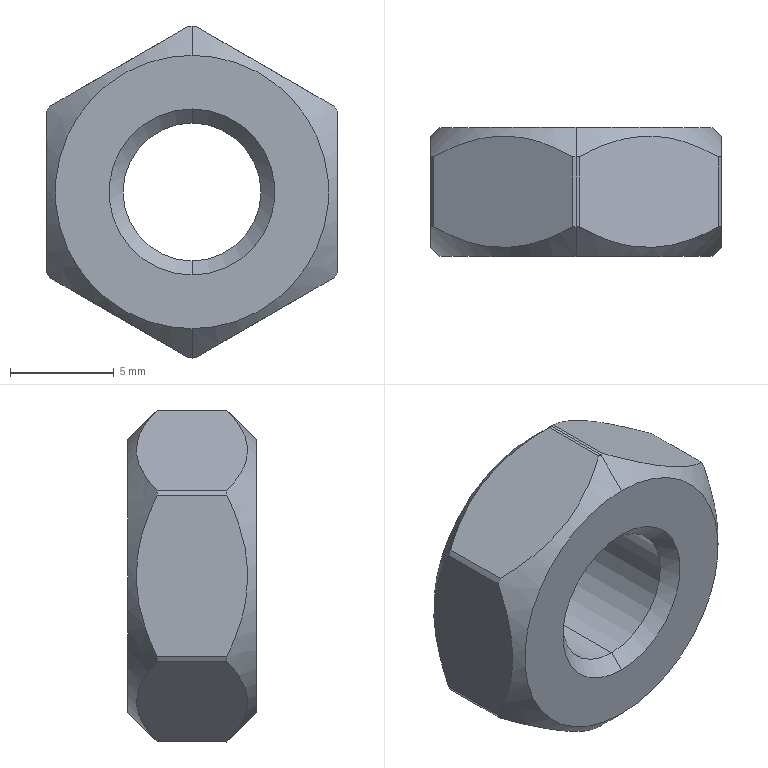Part | SolidWorks | features BaseBody 1 | 1 solid | 23 faces | box 14 x 6.2 x 16 mm | volume 801.096 mm3 | cylinder 9 | plane 8 | cone 6 | commonest cylinder face diameters 16 x7 6.647 x2
STEP:
#1=CARTESIAN_POINT('',(0.,28.776,-3.324));
#2=VERTEX_POINT('',#1);
#3=CARTESIAN_POINT('',(0.,28.776,3.324));
#4=VERTEX_POINT('',#3);
#5=CARTESIAN_POINT('',(0.,28.776,0.));
#6=DIRECTION('',(0.,1.,0.));
#7=DIRECTION('',(0.,0.,1.));
#8=AXIS2_PLACEMENT_3D('',#5,#6,#7);
#9=CIRCLE('',#8,3.324);
#10=EDGE_CURVE('',#2,#4,#9,.T.);
#11=ORIENTED_EDGE('',*,*,#10,.F.);
#12=CARTESIAN_POINT('',(0.,34.3,-3.324));
#13=VERTEX_POINT('',#12);
#14=CARTESIAN_POINT('',(0.,34.3,-3.324));
#15=DIRECTION('',(0.,1.,0.));
#16=VECTOR('',#15,1000.);
#17=LINE('',#14,#16);
#18=EDGE_CURVE('',#2,#13,#17,.T.);
#19=ORIENTED_EDGE('',*,*,#18,.T.);
#20=CARTESIAN_POINT('',(0.,34.3,3.324));
#21=VERTEX_POINT('',#20);
#22=CARTESIAN_POINT('',(0.,34.3,0.));
#23=DIRECTION('',(0.,-1.,0.));
#24=DIRECTION('',(0.,0.,1.));
#25=AXIS2_PLACEMENT_3D('',#22,#23,#24);
#26=CIRCLE('',#25,3.324);
#27=EDGE_CURVE('',#21,#13,#26,.T.);
#28=ORIENTED_EDGE('',*,*,#27,.F.);
#29=CARTESIAN_POINT('',(0.,34.3,3.324));
#30=DIRECTION('',(0.,1.,0.));
#31=VECTOR('',#30,1000.);
#32=LINE('',#29,#31);
#33=EDGE_CURVE('',#4,#21,#32,.T.);
#34=ORIENTED_EDGE('',*,*,#33,.F.);
#35=EDGE_LOOP('',(#11,#19,#28,#34));
#36=FACE_OUTER_BOUND('',#35,.T.);
#37=CARTESIAN_POINT('',(0.,34.3,0.));
#38=DIRECTION('',(0.,1.,0.));
#39=DIRECTION('',(0.,0.,1.));
#40=AXIS2_PLACEMENT_3D('',#37,#38,#39);
#41=CYLINDRICAL_SURFACE('',#40,3.324);
#42=ADVANCED_FACE('',(#36),#41,.F.);
#43=ORIENTED_EDGE('',*,*,#10,.T.);
#44=CARTESIAN_POINT('',(0.,28.1,4.));
#45=VERTEX_POINT('',#44);
#46=CARTESIAN_POINT('',(0.,28.1,4.));
#47=DIRECTION('',(0.,-0.7071,0.7071));
#48=VECTOR('',#47,1000.);
#49=LINE('',#46,#48);
#50=EDGE_CURVE('',#4,#45,#49,.T.);
#51=ORIENTED_EDGE('',*,*,#50,.T.);
#52=CARTESIAN_POINT('',(0.,28.1,-4.));
#53=VERTEX_POINT('',#52);
#54=CARTESIAN_POINT('',(0.,28.1,0.));
#55=DIRECTION('',(0.,1.,0.));
#56=DIRECTION('',(0.,0.,-1.));
#57=AXIS2_PLACEMENT_3D('',#54,#55,#56);
#58=CIRCLE('',#57,4.);
#59=EDGE_CURVE('',#53,#45,#58,.T.);
#60=ORIENTED_EDGE('',*,*,#59,.F.);
#61=CARTESIAN_POINT('',(0.,28.1,-4.));
#62=DIRECTION('',(0.,-0.7071,-0.7071));
#63=VECTOR('',#62,1000.);
#64=LINE('',#61,#63);
#65=EDGE_CURVE('',#2,#53,#64,.T.);
#66=ORIENTED_EDGE('',*,*,#65,.F.);
#67=EDGE_LOOP('',(#43,#51,#60,#66));
#68=FACE_OUTER_BOUND('',#67,.T.);
#69=CARTESIAN_POINT('',(0.,28.1,0.));
#70=DIRECTION('',(0.,-1.,0.));
#71=DIRECTION('',(0.,0.,-1.));
#72=AXIS2_PLACEMENT_3D('',#69,#70,#71);
#73=CONICAL_SURFACE('',#72,4.,0.7854);
#74=ADVANCED_FACE('',(#68),#73,.F.);
#75=CARTESIAN_POINT('',(0.,34.3,-6.586));
#76=VERTEX_POINT('',#75);
#77=CARTESIAN_POINT('',(0.,34.3,6.586));
#78=VERTEX_POINT('',#77);
#79=CARTESIAN_POINT('',(0.,34.3,0.));
#80=DIRECTION('',(0.,-1.,0.));
#81=DIRECTION('',(0.,0.,-1.));
#82=AXIS2_PLACEMENT_3D('',#79,#80,#81);
#83=CIRCLE('',#82,6.586);
#84=EDGE_CURVE('',#76,#78,#83,.T.);
#85=ORIENTED_EDGE('',*,*,#84,.T.);
#86=CARTESIAN_POINT('',(0.,32.886,8.));
#87=VERTEX_POINT('',#86);
#88=CARTESIAN_POINT('',(0.,32.886,8.));
#89=DIRECTION('',(0.,-0.7071,0.7071));
#90=VECTOR('',#89,1000.);
#91=LINE('',#88,#90);
#92=EDGE_CURVE('',#78,#87,#91,.T.);
#93=ORIENTED_EDGE('',*,*,#92,.T.);
#94=CARTESIAN_POINT('',(0.1459,32.886,7.999));
#95=VERTEX_POINT('',#94);
#96=CARTESIAN_POINT('',(0.,32.886,0.));
#97=DIRECTION('',(0.,-1.,0.));
#98=DIRECTION('',(0.,0.,1.));
#99=AXIS2_PLACEMENT_3D('',#96,#97,#98);
#100=CIRCLE('',#99,8.);
#101=EDGE_CURVE('',#95,#87,#100,.T.);
#102=ORIENTED_EDGE('',*,*,#101,.F.);
#103=CARTESIAN_POINT('',(6.854,32.886,4.126));
#104=VERTEX_POINT('',#103);
#105=CARTESIAN_POINT('',(0.1459,32.886,7.999));
#106=CARTESIAN_POINT('',(0.672,33.18,7.695));
#107=CARTESIAN_POINT('',(1.21,33.428,7.385));
#108=CARTESIAN_POINT('',(2.043,33.693,6.903));
#109=CARTESIAN_POINT('',(2.325,33.763,6.74));
#110=CARTESIAN_POINT('',(2.901,33.859,6.408));
#111=CARTESIAN_POINT('',(3.197,33.885,6.237));
#112=CARTESIAN_POINT('',(4.073,33.887,5.731));
#113=CARTESIAN_POINT('',(4.647,33.789,5.4));
#114=CARTESIAN_POINT('',(5.496,33.523,4.91));
#115=CARTESIAN_POINT('',(5.775,33.415,4.749));
#116=CARTESIAN_POINT('',(6.321,33.17,4.433));
#117=CARTESIAN_POINT('',(6.59,33.034,4.278));
#118=CARTESIAN_POINT('',(6.854,32.886,4.126));
#119=B_SPLINE_CURVE_WITH_KNOTS('',3,(#105,#106,#107,#108,#109,#110,#111,#112,#113,#114,#115,#116,#117,#118),.UNSPECIFIED.,.F.,.F.,(4,2,2,2,2,2,4),(0.,0.001996,0.002994,0.003992,0.005988,0.006986,0.007984),.UNSPECIFIED.);
#120=EDGE_CURVE('',#95,#104,#119,.T.);
#121=ORIENTED_EDGE('',*,*,#120,.T.);
#122=CARTESIAN_POINT('',(7.,32.886,3.873));
#123=VERTEX_POINT('',#122);
#124=CARTESIAN_POINT('',(0.,32.886,0.));
#125=DIRECTION('',(0.,-1.,0.));
#126=DIRECTION('',(0.,0.,1.));
#127=AXIS2_PLACEMENT_3D('',#124,#125,#126);
#128=CIRCLE('',#127,8.);
#129=EDGE_CURVE('',#123,#104,#128,.T.);
#130=ORIENTED_EDGE('',*,*,#129,.F.);
#131=CARTESIAN_POINT('',(7.,32.886,-3.873));
#132=VERTEX_POINT('',#131);
#133=CARTESIAN_POINT('',(7.,32.886,3.873));
#134=CARTESIAN_POINT('',(7.,33.18,3.265));
#135=CARTESIAN_POINT('',(7.,33.428,2.645));
#136=CARTESIAN_POINT('',(7.,33.693,1.682));
#137=CARTESIAN_POINT('',(7.,33.763,1.356));
#138=CARTESIAN_POINT('',(7.,33.859,0.6915));
#139=CARTESIAN_POINT('',(7.,33.885,0.3497));
#140=CARTESIAN_POINT('',(7.,33.887,-0.6617));
#141=CARTESIAN_POINT('',(7.,33.789,-1.325));
#142=CARTESIAN_POINT('',(7.,33.523,-2.305));
#143=CARTESIAN_POINT('',(7.,33.415,-2.627));
#144=CARTESIAN_POINT('',(7.,33.17,-3.258));
#145=CARTESIAN_POINT('',(7.,33.034,-3.568));
#146=CARTESIAN_POINT('',(7.,32.886,-3.873));
#147=B_SPLINE_CURVE_WITH_KNOTS('',3,(#133,#134,#135,#136,#137,#138,#139,#140,#141,#142,#143,#144,#145,#146),.UNSPECIFIED.,.F.,.F.,(4,2,2,2,2,2,4),(0.,0.001996,0.002994,0.003992,0.005988,0.006986,0.007984),.UNSPECIFIED.);
#148=EDGE_CURVE('',#123,#132,#147,.T.);
#149=ORIENTED_EDGE('',*,*,#148,.T.);
#150=CARTESIAN_POINT('',(6.854,32.886,-4.126));
#151=VERTEX_POINT('',#150);
#152=CARTESIAN_POINT('',(0.,32.886,0.));
#153=DIRECTION('',(0.,-1.,0.));
#154=DIRECTION('',(0.,0.,1.));
#155=AXIS2_PLACEMENT_3D('',#152,#153,#154);
#156=CIRCLE('',#155,8.);
#157=EDGE_CURVE('',#151,#132,#156,.T.);
#158=ORIENTED_EDGE('',*,*,#157,.F.);
#159=CARTESIAN_POINT('',(0.1459,32.886,-7.999));
#160=VERTEX_POINT('',#159);
#161=CARTESIAN_POINT('',(6.854,32.886,-4.126));
#162=CARTESIAN_POINT('',(6.328,33.18,-4.429));
#163=CARTESIAN_POINT('',(5.79,33.428,-4.74));
#164=CARTESIAN_POINT('',(4.957,33.693,-5.221));
#165=CARTESIAN_POINT('',(4.675,33.763,-5.384));
#166=CARTESIAN_POINT('',(4.099,33.859,-5.716));
#167=CARTESIAN_POINT('',(3.803,33.885,-5.887));
#168=CARTESIAN_POINT('',(2.927,33.887,-6.393));
#169=CARTESIAN_POINT('',(2.353,33.789,-6.724));
#170=CARTESIAN_POINT('',(1.504,33.523,-7.215));
#171=CARTESIAN_POINT('',(1.225,33.415,-7.376));
#172=CARTESIAN_POINT('',(0.6786,33.17,-7.691));
#173=CARTESIAN_POINT('',(0.4103,33.034,-7.846));
#174=CARTESIAN_POINT('',(0.1459,32.886,-7.999));
#175=B_SPLINE_CURVE_WITH_KNOTS('',3,(#161,#162,#163,#164,#165,#166,#167,#168,#169,#170,#171,#172,#173,#174),.UNSPECIFIED.,.F.,.F.,(4,2,2,2,2,2,4),(0.,0.001996,0.002994,0.003992,0.005988,0.006986,0.007984),.UNSPECIFIED.);
#176=EDGE_CURVE('',#151,#160,#175,.T.);
#177=ORIENTED_EDGE('',*,*,#176,.T.);
#178=CARTESIAN_POINT('',(0.,32.886,-8.));
#179=VERTEX_POINT('',#178);
#180=CARTESIAN_POINT('',(0.,32.886,0.));
#181=DIRECTION('',(0.,-1.,0.));
#182=DIRECTION('',(0.,0.,1.));
#183=AXIS2_PLACEMENT_3D('',#180,#181,#182);
#184=CIRCLE('',#183,8.);
#185=EDGE_CURVE('',#179,#160,#184,.T.);
#186=ORIENTED_EDGE('',*,*,#185,.F.);
#187=CARTESIAN_POINT('',(0.,32.886,-8.));
#188=DIRECTION('',(0.,-0.7071,-0.7071));
#189=VECTOR('',#188,1000.);
#190=LINE('',#187,#189);
#191=EDGE_CURVE('',#76,#179,#190,.T.);
#192=ORIENTED_EDGE('',*,*,#191,.F.);
#193=EDGE_LOOP('',(#85,#93,#102,#121,#130,#149,#158,#177,#186,#192));
#194=FACE_OUTER_BOUND('',#193,.T.);
#195=CARTESIAN_POINT('',(0.,32.886,0.));
#196=DIRECTION('',(0.,-1.,0.));
#197=DIRECTION('',(0.,0.,-1.));
#198=AXIS2_PLACEMENT_3D('',#195,#196,#197);
#199=CONICAL_SURFACE('',#198,8.,0.7854);
#200=ADVANCED_FACE('',(#194),#199,.T.);
#201=CARTESIAN_POINT('',(0.,28.1,6.586));
#202=VERTEX_POINT('',#201);
#203=CARTESIAN_POINT('',(0.,28.1,-6.586));
#204=VERTEX_POINT('',#203);
#205=CARTESIAN_POINT('',(0.,28.1,0.));
#206=DIRECTION('',(0.,1.,0.));
#207=DIRECTION('',(0.,0.,1.));
#208=AXIS2_PLACEMENT_3D('',#205,#206,#207);
#209=CIRCLE('',#208,6.586);
#210=EDGE_CURVE('',#202,#204,#209,.T.);
#211=ORIENTED_EDGE('',*,*,#210,.T.);
#212=CARTESIAN_POINT('',(0.,29.514,-8.));
#213=VERTEX_POINT('',#212);
#214=CARTESIAN_POINT('',(0.,29.514,-8.));
#215=DIRECTION('',(0.,0.7071,-0.7071));
#216=VECTOR('',#215,1000.);
#217=LINE('',#214,#216);
#218=EDGE_CURVE('',#204,#213,#217,.T.);
#219=ORIENTED_EDGE('',*,*,#218,.T.);
#220=CARTESIAN_POINT('',(0.1459,29.514,-7.999));
#221=VERTEX_POINT('',#220);
#222=CARTESIAN_POINT('',(0.,29.514,0.));
#223=DIRECTION('',(0.,1.,0.));
#224=DIRECTION('',(0.,0.,1.));
#225=AXIS2_PLACEMENT_3D('',#222,#223,#224);
#226=CIRCLE('',#225,8.);
#227=EDGE_CURVE('',#221,#213,#226,.T.);
#228=ORIENTED_EDGE('',*,*,#227,.F.);
#229=CARTESIAN_POINT('',(6.854,29.514,-4.126));
#230=VERTEX_POINT('',#229);
#231=CARTESIAN_POINT('',(0.1459,29.514,-7.999));
#232=CARTESIAN_POINT('',(0.672,29.22,-7.695));
#233=CARTESIAN_POINT('',(1.21,28.972,-7.385));
#234=CARTESIAN_POINT('',(2.043,28.707,-6.903));
#235=CARTESIAN_POINT('',(2.325,28.637,-6.74));
#236=CARTESIAN_POINT('',(2.901,28.541,-6.408));
#237=CARTESIAN_POINT('',(3.197,28.515,-6.237));
#238=CARTESIAN_POINT('',(4.073,28.513,-5.731));
#239=CARTESIAN_POINT('',(4.647,28.611,-5.4));
#240=CARTESIAN_POINT('',(5.496,28.877,-4.91));
#241=CARTESIAN_POINT('',(5.775,28.985,-4.749));
#242=CARTESIAN_POINT('',(6.321,29.23,-4.433));
#243=CARTESIAN_POINT('',(6.59,29.366,-4.278));
#244=CARTESIAN_POINT('',(6.854,29.514,-4.126));
#245=B_SPLINE_CURVE_WITH_KNOTS('',3,(#231,#232,#233,#234,#235,#236,#237,#238,#239,#240,#241,#242,#243,#244),.UNSPECIFIED.,.F.,.F.,(4,2,2,2,2,2,4),(0.,0.001996,0.002994,0.003992,0.005988,0.006986,0.007984),.UNSPECIFIED.);
#246=EDGE_CURVE('',#221,#230,#245,.T.);
#247=ORIENTED_EDGE('',*,*,#246,.T.);
#248=CARTESIAN_POINT('',(7.,29.514,-3.873));
#249=VERTEX_POINT('',#248);
#250=CARTESIAN_POINT('',(0.,29.514,0.));
#251=DIRECTION('',(0.,1.,0.));
#252=DIRECTION('',(0.,0.,1.));
#253=AXIS2_PLACEMENT_3D('',#250,#251,#252);
#254=CIRCLE('',#253,8.);
#255=EDGE_CURVE('',#249,#230,#254,.T.);
#256=ORIENTED_EDGE('',*,*,#255,.F.);
#257=CARTESIAN_POINT('',(7.,29.514,3.873));
#258=VERTEX_POINT('',#257);
#259=CARTESIAN_POINT('',(7.,29.514,-3.873));
#260=CARTESIAN_POINT('',(7.,29.22,-3.265));
#261=CARTESIAN_POINT('',(7.,28.972,-2.645));
#262=CARTESIAN_POINT('',(7.,28.707,-1.682));
#263=CARTESIAN_POINT('',(7.,28.637,-1.356));
#264=CARTESIAN_POINT('',(7.,28.541,-0.6915));
#265=CARTESIAN_POINT('',(7.,28.515,-0.3497));
#266=CARTESIAN_POINT('',(7.,28.513,0.6617));
#267=CARTESIAN_POINT('',(7.,28.611,1.325));
#268=CARTESIAN_POINT('',(7.,28.877,2.305));
#269=CARTESIAN_POINT('',(7.,28.985,2.627));
#270=CARTESIAN_POINT('',(7.,29.23,3.258));
#271=CARTESIAN_POINT('',(7.,29.366,3.568));
#272=CARTESIAN_POINT('',(7.,29.514,3.873));
#273=B_SPLINE_CURVE_WITH_KNOTS('',3,(#259,#260,#261,#262,#263,#264,#265,#266,#267,#268,#269,#270,#271,#272),.UNSPECIFIED.,.F.,.F.,(4,2,2,2,2,2,4),(0.,0.001996,0.002994,0.003992,0.005988,0.006986,0.007984),.UNSPECIFIED.);
#274=EDGE_CURVE('',#249,#258,#273,.T.);
#275=ORIENTED_EDGE('',*,*,#274,.T.);
#276=CARTESIAN_POINT('',(6.854,29.514,4.126));
#277=VERTEX_POINT('',#276);
#278=CARTESIAN_POINT('',(0.,29.514,0.));
#279=DIRECTION('',(0.,1.,0.));
#280=DIRECTION('',(0.,0.,1.));
#281=AXIS2_PLACEMENT_3D('',#278,#279,#280);
#282=CIRCLE('',#281,8.);
#283=EDGE_CURVE('',#277,#258,#282,.T.);
#284=ORIENTED_EDGE('',*,*,#283,.F.);
#285=CARTESIAN_POINT('',(0.1459,29.514,7.999));
#286=VERTEX_POINT('',#285);
#287=CARTESIAN_POINT('',(6.854,29.514,4.126));
#288=CARTESIAN_POINT('',(6.328,29.22,4.429));
#289=CARTESIAN_POINT('',(5.79,28.972,4.74));
#290=CARTESIAN_POINT('',(4.957,28.707,5.221));
#291=CARTESIAN_POINT('',(4.675,28.637,5.384));
#292=CARTESIAN_POINT('',(4.099,28.541,5.716));
#293=CARTESIAN_POINT('',(3.803,28.515,5.887));
#294=CARTESIAN_POINT('',(2.927,28.513,6.393));
#295=CARTESIAN_POINT('',(2.353,28.611,6.724));
#296=CARTESIAN_POINT('',(1.504,28.877,7.215));
#297=CARTESIAN_POINT('',(1.225,28.985,7.376));
#298=CARTESIAN_POINT('',(0.6786,29.23,7.691));
#299=CARTESIAN_POINT('',(0.4103,29.366,7.846));
#300=CARTESIAN_POINT('',(0.1459,29.514,7.999));
#301=B_SPLINE_CURVE_WITH_KNOTS('',3,(#287,#288,#289,#290,#291,#292,#293,#294,#295,#296,#297,#298,#299,#300),.UNSPECIFIED.,.F.,.F.,(4,2,2,2,2,2,4),(0.,0.001996,0.002994,0.003992,0.005988,0.006986,0.007984),.UNSPECIFIED.);
#302=EDGE_CURVE('',#277,#286,#301,.T.);
#303=ORIENTED_EDGE('',*,*,#302,.T.);
#304=CARTESIAN_POINT('',(0.,29.514,8.));
#305=VERTEX_POINT('',#304);
#306=CARTESIAN_POINT('',(0.,29.514,0.));
#307=DIRECTION('',(0.,1.,0.));
#308=DIRECTION('',(0.,0.,1.));
#309=AXIS2_PLACEMENT_3D('',#306,#307,#308);
#310=CIRCLE('',#309,8.);
#311=EDGE_CURVE('',#305,#286,#310,.T.);
#312=ORIENTED_EDGE('',*,*,#311,.F.);
#313=CARTESIAN_POINT('',(0.,29.514,8.));
#314=DIRECTION('',(0.,0.7071,0.7071));
#315=VECTOR('',#314,1000.);
#316=LINE('',#313,#315);
#317=EDGE_CURVE('',#202,#305,#316,.T.);
#318=ORIENTED_EDGE('',*,*,#317,.F.);
#319=EDGE_LOOP('',(#211,#219,#228,#247,#256,#275,#284,#303,#312,#318));
#320=FACE_OUTER_BOUND('',#319,.T.);
#321=CARTESIAN_POINT('',(0.,29.514,0.));
#322=DIRECTION('',(0.,1.,0.));
#323=DIRECTION('',(0.,0.,1.));
#324=AXIS2_PLACEMENT_3D('',#321,#322,#323);
#325=CONICAL_SURFACE('',#324,8.,0.7854);
#326=ADVANCED_FACE('',(#320),#325,.T.);
#327=CARTESIAN_POINT('',(-0.1459,29.514,7.999));
#328=VERTEX_POINT('',#327);
#329=CARTESIAN_POINT('',(0.,29.514,0.));
#330=DIRECTION('',(0.,1.,0.));
#331=DIRECTION('',(0.,0.,1.));
#332=AXIS2_PLACEMENT_3D('',#329,#330,#331);
#333=CIRCLE('',#332,8.);
#334=EDGE_CURVE('',#328,#305,#333,.T.);
#335=ORIENTED_EDGE('',*,*,#334,.T.);
#336=CARTESIAN_POINT('',(0.,34.3,8.));
#337=DIRECTION('',(0.,1.,0.));
#338=VECTOR('',#337,1000.);
#339=LINE('',#336,#338);
#340=EDGE_CURVE('',#305,#87,#339,.T.);
#341=ORIENTED_EDGE('',*,*,#340,.T.);
#342=CARTESIAN_POINT('',(-0.1459,32.886,7.999));
#343=VERTEX_POINT('',#342);
#344=CARTESIAN_POINT('',(0.,32.886,0.));
#345=DIRECTION('',(0.,-1.,0.));
#346=DIRECTION('',(0.,0.,1.));
#347=AXIS2_PLACEMENT_3D('',#344,#345,#346);
#348=CIRCLE('',#347,8.);
#349=EDGE_CURVE('',#87,#343,#348,.T.);
#350=ORIENTED_EDGE('',*,*,#349,.T.);
#351=CARTESIAN_POINT('',(-0.1459,34.3,7.999));
#352=DIRECTION('',(0.,-1.,0.));
#353=VECTOR('',#352,1000.);
#354=LINE('',#351,#353);
#355=EDGE_CURVE('',#343,#328,#354,.T.);
#356=ORIENTED_EDGE('',*,*,#355,.T.);
#357=EDGE_LOOP('',(#335,#341,#350,#356));
#358=FACE_OUTER_BOUND('',#357,.T.);
#359=CARTESIAN_POINT('',(0.,34.3,0.));
#360=DIRECTION('',(0.,1.,0.));
#361=DIRECTION('',(0.,0.,1.));
#362=AXIS2_PLACEMENT_3D('',#359,#360,#361);
#363=CYLINDRICAL_SURFACE('',#362,8.);
#364=ADVANCED_FACE('',(#358),#363,.T.);
#365=ORIENTED_EDGE('',*,*,#18,.F.);
#366=CARTESIAN_POINT('',(0.,28.776,0.));
#367=DIRECTION('',(0.,1.,0.));
#368=DIRECTION('',(0.,0.,1.));
#369=AXIS2_PLACEMENT_3D('',#366,#367,#368);
#370=CIRCLE('',#369,3.324);
#371=EDGE_CURVE('',#4,#2,#370,.T.);
#372=ORIENTED_EDGE('',*,*,#371,.F.);
#373=ORIENTED_EDGE('',*,*,#33,.T.);
#374=CARTESIAN_POINT('',(0.,34.3,0.));
#375=DIRECTION('',(0.,-1.,0.));
#376=DIRECTION('',(0.,0.,1.));
#377=AXIS2_PLACEMENT_3D('',#374,#375,#376);
#378=CIRCLE('',#377,3.324);
#379=EDGE_CURVE('',#13,#21,#378,.T.);
#380=ORIENTED_EDGE('',*,*,#379,.F.);
#381=EDGE_LOOP('',(#365,#372,#373,#380));
#382=FACE_OUTER_BOUND('',#381,.T.);
#383=CARTESIAN_POINT('',(0.,34.3,0.));
#384=DIRECTION('',(0.,1.,0.));
#385=DIRECTION('',(0.,0.,1.));
#386=AXIS2_PLACEMENT_3D('',#383,#384,#385);
#387=CYLINDRICAL_SURFACE('',#386,3.324);
#388=ADVANCED_FACE('',(#382),#387,.F.);
#389=ORIENTED_EDGE('',*,*,#50,.F.);
#390=ORIENTED_EDGE('',*,*,#371,.T.);
#391=ORIENTED_EDGE('',*,*,#65,.T.);
#392=CARTESIAN_POINT('',(0.,28.1,0.));
#393=DIRECTION('',(0.,1.,0.));
#394=DIRECTION('',(0.,0.,-1.));
#395=AXIS2_PLACEMENT_3D('',#392,#393,#394);
#396=CIRCLE('',#395,4.);
#397=EDGE_CURVE('',#45,#53,#396,.T.);
#398=ORIENTED_EDGE('',*,*,#397,.F.);
#399=EDGE_LOOP('',(#389,#390,#391,#398));
#400=FACE_OUTER_BOUND('',#399,.T.);
#401=CARTESIAN_POINT('',(0.,28.1,0.));
#402=DIRECTION('',(0.,-1.,0.));
#403=DIRECTION('',(0.,0.,-1.));
#404=AXIS2_PLACEMENT_3D('',#401,#402,#403);
#405=CONICAL_SURFACE('',#404,4.,0.7854);
#406=ADVANCED_FACE('',(#400),#405,.F.);
#407=ORIENTED_EDGE('',*,*,#84,.F.);
#408=CARTESIAN_POINT('',(0.,34.3,0.));
#409=DIRECTION('',(0.,-1.,0.));
#410=DIRECTION('',(0.,0.,-1.));
#411=AXIS2_PLACEMENT_3D('',#408,#409,#410);
#412=CIRCLE('',#411,6.586);
#413=EDGE_CURVE('',#78,#76,#412,.T.);
#414=ORIENTED_EDGE('',*,*,#413,.F.);
#415=EDGE_LOOP('',(#407,#414));
#416=FACE_OUTER_BOUND('',#415,.T.);
#417=ORIENTED_EDGE('',*,*,#27,.T.);
#418=ORIENTED_EDGE('',*,*,#379,.T.);
#419=EDGE_LOOP('',(#417,#418));
#420=FACE_BOUND('',#419,.T.);
#421=CARTESIAN_POINT('',(0.,34.3,6.586));
#422=DIRECTION('',(0.,-1.,0.));
#423=DIRECTION('',(0.,0.,-1.));
#424=AXIS2_PLACEMENT_3D('',#421,#422,#423);
#425=PLANE('',#424);
#426=ADVANCED_FACE('',(#416,#420),#425,.F.);
#427=ORIENTED_EDGE('',*,*,#210,.F.);
#428=CARTESIAN_POINT('',(0.,28.1,0.));
#429=DIRECTION('',(0.,1.,0.));
#430=DIRECTION('',(0.,0.,1.));
#431=AXIS2_PLACEMENT_3D('',#428,#429,#430);
#432=CIRCLE('',#431,6.586);
#433=EDGE_CURVE('',#204,#202,#432,.T.);
#434=ORIENTED_EDGE('',*,*,#433,.F.);
#435=EDGE_LOOP('',(#427,#434));
#436=FACE_OUTER_BOUND('',#435,.T.);
#437=ORIENTED_EDGE('',*,*,#59,.T.);
#438=ORIENTED_EDGE('',*,*,#397,.T.);
#439=EDGE_LOOP('',(#437,#438));
#440=FACE_BOUND('',#439,.T.);
#441=CARTESIAN_POINT('',(0.,28.1,0.));
#442=DIRECTION('',(0.,1.,0.));
#443=DIRECTION('',(0.,0.,1.));
#444=AXIS2_PLACEMENT_3D('',#441,#442,#443);
#445=PLANE('',#444);
#446=ADVANCED_FACE('',(#436,#440),#445,.F.);
#447=ORIENTED_EDGE('',*,*,#92,.F.);
#448=ORIENTED_EDGE('',*,*,#413,.T.);
#449=ORIENTED_EDGE('',*,*,#191,.T.);
#450=CARTESIAN_POINT('',(-0.1459,32.886,-7.999));
#451=VERTEX_POINT('',#450);
#452=CARTESIAN_POINT('',(0.,32.886,0.));
#453=DIRECTION('',(0.,-1.,0.));
#454=DIRECTION('',(0.,0.,1.));
#455=AXIS2_PLACEMENT_3D('',#452,#453,#454);
#456=CIRCLE('',#455,8.);
#457=EDGE_CURVE('',#451,#179,#456,.T.);
#458=ORIENTED_EDGE('',*,*,#457,.F.);
#459=CARTESIAN_POINT('',(-6.854,32.886,-4.126));
#460=VERTEX_POINT('',#459);
#461=CARTESIAN_POINT('',(-0.1459,32.886,-7.999));
#462=CARTESIAN_POINT('',(-0.672,33.18,-7.695));
#463=CARTESIAN_POINT('',(-1.21,33.428,-7.385));
#464=CARTESIAN_POINT('',(-2.043,33.693,-6.903));
#465=CARTESIAN_POINT('',(-2.325,33.763,-6.74));
#466=CARTESIAN_POINT('',(-2.901,33.859,-6.408));
#467=CARTESIAN_POINT('',(-3.197,33.885,-6.237));
#468=CARTESIAN_POINT('',(-4.073,33.887,-5.731));
#469=CARTESIAN_POINT('',(-4.647,33.789,-5.4));
#470=CARTESIAN_POINT('',(-5.496,33.523,-4.91));
#471=CARTESIAN_POINT('',(-5.775,33.415,-4.749));
#472=CARTESIAN_POINT('',(-6.321,33.17,-4.433));
#473=CARTESIAN_POINT('',(-6.59,33.034,-4.278));
#474=CARTESIAN_POINT('',(-6.854,32.886,-4.126));
#475=B_SPLINE_CURVE_WITH_KNOTS('',3,(#461,#462,#463,#464,#465,#466,#467,#468,#469,#470,#471,#472,#473,#474),.UNSPECIFIED.,.F.,.F.,(4,2,2,2,2,2,4),(0.,0.001996,0.002994,0.003992,0.005988,0.006986,0.007984),.UNSPECIFIED.);
#476=EDGE_CURVE('',#451,#460,#475,.T.);
#477=ORIENTED_EDGE('',*,*,#476,.T.);
#478=CARTESIAN_POINT('',(-7.,32.886,-3.873));
#479=VERTEX_POINT('',#478);
#480=CARTESIAN_POINT('',(0.,32.886,0.));
#481=DIRECTION('',(0.,-1.,0.));
#482=DIRECTION('',(0.,0.,1.));
#483=AXIS2_PLACEMENT_3D('',#480,#481,#482);
#484=CIRCLE('',#483,8.);
#485=EDGE_CURVE('',#479,#460,#484,.T.);
#486=ORIENTED_EDGE('',*,*,#485,.F.);
#487=CARTESIAN_POINT('',(-7.,32.886,3.873));
#488=VERTEX_POINT('',#487);
#489=CARTESIAN_POINT('',(-7.,32.886,-3.873));
#490=CARTESIAN_POINT('',(-7.,33.18,-3.265));
#491=CARTESIAN_POINT('',(-7.,33.428,-2.645));
#492=CARTESIAN_POINT('',(-7.,33.693,-1.682));
#493=CARTESIAN_POINT('',(-7.,33.763,-1.356));
#494=CARTESIAN_POINT('',(-7.,33.859,-0.6915));
#495=CARTESIAN_POINT('',(-7.,33.885,-0.3497));
#496=CARTESIAN_POINT('',(-7.,33.887,0.6617));
#497=CARTESIAN_POINT('',(-7.,33.789,1.325));
#498=CARTESIAN_POINT('',(-7.,33.523,2.305));
#499=CARTESIAN_POINT('',(-7.,33.415,2.627));
#500=CARTESIAN_POINT('',(-7.,33.17,3.258));
#501=CARTESIAN_POINT('',(-7.,33.034,3.568));
#502=CARTESIAN_POINT('',(-7.,32.886,3.873));
#503=B_SPLINE_CURVE_WITH_KNOTS('',3,(#489,#490,#491,#492,#493,#494,#495,#496,#497,#498,#499,#500,#501,#502),.UNSPECIFIED.,.F.,.F.,(4,2,2,2,2,2,4),(0.,0.001996,0.002994,0.003992,0.005988,0.006986,0.007984),.UNSPECIFIED.);
#504=EDGE_CURVE('',#479,#488,#503,.T.);
#505=ORIENTED_EDGE('',*,*,#504,.T.);
#506=CARTESIAN_POINT('',(-6.854,32.886,4.126));
#507=VERTEX_POINT('',#506);
#508=CARTESIAN_POINT('',(0.,32.886,0.));
#509=DIRECTION('',(0.,-1.,0.));
#510=DIRECTION('',(0.,0.,1.));
#511=AXIS2_PLACEMENT_3D('',#508,#509,#510);
#512=CIRCLE('',#511,8.);
#513=EDGE_CURVE('',#507,#488,#512,.T.);
#514=ORIENTED_EDGE('',*,*,#513,.F.);
#515=CARTESIAN_POINT('',(-6.854,32.886,4.126));
#516=CARTESIAN_POINT('',(-6.328,33.18,4.429));
#517=CARTESIAN_POINT('',(-5.79,33.428,4.74));
#518=CARTESIAN_POINT('',(-4.957,33.693,5.221));
#519=CARTESIAN_POINT('',(-4.675,33.763,5.384));
#520=CARTESIAN_POINT('',(-4.099,33.859,5.716));
#521=CARTESIAN_POINT('',(-3.803,33.885,5.887));
#522=CARTESIAN_POINT('',(-2.927,33.887,6.393));
#523=CARTESIAN_POINT('',(-2.353,33.789,6.724));
#524=CARTESIAN_POINT('',(-1.504,33.523,7.215));
#525=CARTESIAN_POINT('',(-1.225,33.415,7.376));
#526=CARTESIAN_POINT('',(-0.6786,33.17,7.691));
#527=CARTESIAN_POINT('',(-0.4103,33.034,7.846));
#528=CARTESIAN_POINT('',(-0.1459,32.886,7.999));
#529=B_SPLINE_CURVE_WITH_KNOTS('',3,(#515,#516,#517,#518,#519,#520,#521,#522,#523,#524,#525,#526,#527,#528),.UNSPECIFIED.,.F.,.F.,(4,2,2,2,2,2,4),(0.,0.001996,0.002994,0.003992,0.005988,0.006986,0.007984),.UNSPECIFIED.);
#530=EDGE_CURVE('',#507,#343,#529,.T.);
#531=ORIENTED_EDGE('',*,*,#530,.T.);
#532=ORIENTED_EDGE('',*,*,#349,.F.);
#533=EDGE_LOOP('',(#447,#448,#449,#458,#477,#486,#505,#514,#531,#532));
#534=FACE_OUTER_BOUND('',#533,.T.);
#535=CARTESIAN_POINT('',(0.,32.886,0.));
#536=DIRECTION('',(0.,-1.,0.));
#537=DIRECTION('',(0.,0.,-1.));
#538=AXIS2_PLACEMENT_3D('',#535,#536,#537);
#539=CONICAL_SURFACE('',#538,8.,0.7854);
#540=ADVANCED_FACE('',(#534),#539,.T.);
#541=ORIENTED_EDGE('',*,*,#218,.F.);
#542=ORIENTED_EDGE('',*,*,#433,.T.);
#543=ORIENTED_EDGE('',*,*,#317,.T.);
#544=ORIENTED_EDGE('',*,*,#334,.F.);
#545=CARTESIAN_POINT('',(-6.854,29.514,4.126));
#546=VERTEX_POINT('',#545);
#547=CARTESIAN_POINT('',(-0.1459,29.514,7.999));
#548=CARTESIAN_POINT('',(-0.672,29.22,7.695));
#549=CARTESIAN_POINT('',(-1.21,28.972,7.385));
#550=CARTESIAN_POINT('',(-2.043,28.707,6.903));
#551=CARTESIAN_POINT('',(-2.325,28.637,6.74));
#552=CARTESIAN_POINT('',(-2.901,28.541,6.408));
#553=CARTESIAN_POINT('',(-3.197,28.515,6.237));
#554=CARTESIAN_POINT('',(-4.073,28.513,5.731));
#555=CARTESIAN_POINT('',(-4.647,28.611,5.4));
#556=CARTESIAN_POINT('',(-5.496,28.877,4.91));
#557=CARTESIAN_POINT('',(-5.775,28.985,4.749));
#558=CARTESIAN_POINT('',(-6.321,29.23,4.433));
#559=CARTESIAN_POINT('',(-6.59,29.366,4.278));
#560=CARTESIAN_POINT('',(-6.854,29.514,4.126));
#561=B_SPLINE_CURVE_WITH_KNOTS('',3,(#547,#548,#549,#550,#551,#552,#553,#554,#555,#556,#557,#558,#559,#560),.UNSPECIFIED.,.F.,.F.,(4,2,2,2,2,2,4),(0.,0.001996,0.002994,0.003992,0.005988,0.006986,0.007984),.UNSPECIFIED.);
#562=EDGE_CURVE('',#328,#546,#561,.T.);
#563=ORIENTED_EDGE('',*,*,#562,.T.);
#564=CARTESIAN_POINT('',(-7.,29.514,3.873));
#565=VERTEX_POINT('',#564);
#566=CARTESIAN_POINT('',(0.,29.514,0.));
#567=DIRECTION('',(0.,1.,0.));
#568=DIRECTION('',(0.,0.,1.));
#569=AXIS2_PLACEMENT_3D('',#566,#567,#568);
#570=CIRCLE('',#569,8.);
#571=EDGE_CURVE('',#565,#546,#570,.T.);
#572=ORIENTED_EDGE('',*,*,#571,.F.);
#573=CARTESIAN_POINT('',(-7.,29.514,-3.873));
#574=VERTEX_POINT('',#573);
#575=CARTESIAN_POINT('',(-7.,29.514,3.873));
#576=CARTESIAN_POINT('',(-7.,29.22,3.265));
#577=CARTESIAN_POINT('',(-7.,28.972,2.645));
#578=CARTESIAN_POINT('',(-7.,28.707,1.682));
#579=CARTESIAN_POINT('',(-7.,28.637,1.356));
#580=CARTESIAN_POINT('',(-7.,28.541,0.6915));
#581=CARTESIAN_POINT('',(-7.,28.515,0.3497));
#582=CARTESIAN_POINT('',(-7.,28.513,-0.6617));
#583=CARTESIAN_POINT('',(-7.,28.611,-1.325));
#584=CARTESIAN_POINT('',(-7.,28.877,-2.305));
#585=CARTESIAN_POINT('',(-7.,28.985,-2.627));
#586=CARTESIAN_POINT('',(-7.,29.23,-3.258));
#587=CARTESIAN_POINT('',(-7.,29.366,-3.568));
#588=CARTESIAN_POINT('',(-7.,29.514,-3.873));
#589=B_SPLINE_CURVE_WITH_KNOTS('',3,(#575,#576,#577,#578,#579,#580,#581,#582,#583,#584,#585,#586,#587,#588),.UNSPECIFIED.,.F.,.F.,(4,2,2,2,2,2,4),(0.,0.001996,0.002994,0.003992,0.005988,0.006986,0.007984),.UNSPECIFIED.);
#590=EDGE_CURVE('',#565,#574,#589,.T.);
#591=ORIENTED_EDGE('',*,*,#590,.T.);
#592=CARTESIAN_POINT('',(-6.854,29.514,-4.126));
#593=VERTEX_POINT('',#592);
#594=CARTESIAN_POINT('',(0.,29.514,0.));
#595=DIRECTION('',(0.,1.,0.));
#596=DIRECTION('',(0.,0.,1.));
#597=AXIS2_PLACEMENT_3D('',#594,#595,#596);
#598=CIRCLE('',#597,8.);
#599=EDGE_CURVE('',#593,#574,#598,.T.);
#600=ORIENTED_EDGE('',*,*,#599,.F.);
#601=CARTESIAN_POINT('',(-0.1459,29.514,-7.999));
#602=VERTEX_POINT('',#601);
#603=CARTESIAN_POINT('',(-6.854,29.514,-4.126));
#604=CARTESIAN_POINT('',(-6.328,29.22,-4.429));
#605=CARTESIAN_POINT('',(-5.79,28.972,-4.74));
#606=CARTESIAN_POINT('',(-4.957,28.707,-5.221));
#607=CARTESIAN_POINT('',(-4.675,28.637,-5.384));
#608=CARTESIAN_POINT('',(-4.099,28.541,-5.716));
#609=CARTESIAN_POINT('',(-3.803,28.515,-5.887));
#610=CARTESIAN_POINT('',(-2.927,28.513,-6.393));
#611=CARTESIAN_POINT('',(-2.353,28.611,-6.724));
#612=CARTESIAN_POINT('',(-1.504,28.877,-7.215));
#613=CARTESIAN_POINT('',(-1.225,28.985,-7.376));
#614=CARTESIAN_POINT('',(-0.6786,29.23,-7.691));
#615=CARTESIAN_POINT('',(-0.4103,29.366,-7.846));
#616=CARTESIAN_POINT('',(-0.1459,29.514,-7.999));
#617=B_SPLINE_CURVE_WITH_KNOTS('',3,(#603,#604,#605,#606,#607,#608,#609,#610,#611,#612,#613,#614,#615,#616),.UNSPECIFIED.,.F.,.F.,(4,2,2,2,2,2,4),(0.,0.001996,0.002994,0.003992,0.005988,0.006986,0.007984),.UNSPECIFIED.);
#618=EDGE_CURVE('',#593,#602,#617,.T.);
#619=ORIENTED_EDGE('',*,*,#618,.T.);
#620=CARTESIAN_POINT('',(0.,29.514,0.));
#621=DIRECTION('',(0.,1.,0.));
#622=DIRECTION('',(0.,0.,1.));
#623=AXIS2_PLACEMENT_3D('',#620,#621,#622);
#624=CIRCLE('',#623,8.);
#625=EDGE_CURVE('',#213,#602,#624,.T.);
#626=ORIENTED_EDGE('',*,*,#625,.F.);
#627=EDGE_LOOP('',(#541,#542,#543,#544,#563,#572,#591,#600,#619,#626));
#628=FACE_OUTER_BOUND('',#627,.T.);
#629=CARTESIAN_POINT('',(0.,29.514,0.));
#630=DIRECTION('',(0.,1.,0.));
#631=DIRECTION('',(0.,0.,1.));
#632=AXIS2_PLACEMENT_3D('',#629,#630,#631);
#633=CONICAL_SURFACE('',#632,8.,0.7854);
#634=ADVANCED_FACE('',(#628),#633,.T.);
#635=ORIENTED_EDGE('',*,*,#476,.F.);
#636=CARTESIAN_POINT('',(-0.1459,34.3,-7.999));
#637=DIRECTION('',(0.,1.,0.));
#638=VECTOR('',#637,1000.);
#639=LINE('',#636,#638);
#640=EDGE_CURVE('',#602,#451,#639,.T.);
#641=ORIENTED_EDGE('',*,*,#640,.F.);
#642=ORIENTED_EDGE('',*,*,#618,.F.);
#643=CARTESIAN_POINT('',(-6.854,34.3,-4.126));
#644=DIRECTION('',(0.,-1.,0.));
#645=VECTOR('',#644,1000.);
#646=LINE('',#643,#645);
#647=EDGE_CURVE('',#460,#593,#646,.T.);
#648=ORIENTED_EDGE('',*,*,#647,.F.);
#649=EDGE_LOOP('',(#635,#641,#642,#648));
#650=FACE_OUTER_BOUND('',#649,.T.);
#651=CARTESIAN_POINT('',(0.,34.3,-8.083));
#652=DIRECTION('',(0.5,0.,0.866));
#653=DIRECTION('',(0.866,0.,-0.5));
#654=AXIS2_PLACEMENT_3D('',#651,#652,#653);
#655=PLANE('',#654);
#656=ADVANCED_FACE('',(#650),#655,.F.);
#657=ORIENTED_EDGE('',*,*,#176,.F.);
#658=CARTESIAN_POINT('',(6.854,34.3,-4.126));
#659=DIRECTION('',(0.,1.,0.));
#660=VECTOR('',#659,1000.);
#661=LINE('',#658,#660);
#662=EDGE_CURVE('',#230,#151,#661,.T.);
#663=ORIENTED_EDGE('',*,*,#662,.F.);
#664=ORIENTED_EDGE('',*,*,#246,.F.);
#665=CARTESIAN_POINT('',(0.1459,34.3,-7.999));
#666=DIRECTION('',(0.,-1.,0.));
#667=VECTOR('',#666,1000.);
#668=LINE('',#665,#667);
#669=EDGE_CURVE('',#160,#221,#668,.T.);
#670=ORIENTED_EDGE('',*,*,#669,.F.);
#671=EDGE_LOOP('',(#657,#663,#664,#670));
#672=FACE_OUTER_BOUND('',#671,.T.);
#673=CARTESIAN_POINT('',(7.,34.3,-4.041));
#674=DIRECTION('',(-0.5,0.,0.866));
#675=DIRECTION('',(0.866,0.,0.5));
#676=AXIS2_PLACEMENT_3D('',#673,#674,#675);
#677=PLANE('',#676);
#678=ADVANCED_FACE('',(#672),#677,.F.);
#679=ORIENTED_EDGE('',*,*,#148,.F.);
#680=CARTESIAN_POINT('',(7.,34.3,3.873));
#681=DIRECTION('',(0.,1.,0.));
#682=VECTOR('',#681,1000.);
#683=LINE('',#680,#682);
#684=EDGE_CURVE('',#258,#123,#683,.T.);
#685=ORIENTED_EDGE('',*,*,#684,.F.);
#686=ORIENTED_EDGE('',*,*,#274,.F.);
#687=CARTESIAN_POINT('',(7.,34.3,-3.873));
#688=DIRECTION('',(0.,-1.,0.));
#689=VECTOR('',#688,1000.);
#690=LINE('',#687,#689);
#691=EDGE_CURVE('',#132,#249,#690,.T.);
#692=ORIENTED_EDGE('',*,*,#691,.F.);
#693=EDGE_LOOP('',(#679,#685,#686,#692));
#694=FACE_OUTER_BOUND('',#693,.T.);
#695=CARTESIAN_POINT('',(7.,34.3,4.041));
#696=DIRECTION('',(-1.,0.,0.));
#697=DIRECTION('',(0.,0.,1.));
#698=AXIS2_PLACEMENT_3D('',#695,#696,#697);
#699=PLANE('',#698);
#700=ADVANCED_FACE('',(#694),#699,.F.);
#701=ORIENTED_EDGE('',*,*,#120,.F.);
#702=CARTESIAN_POINT('',(0.1459,34.3,7.999));
#703=DIRECTION('',(0.,1.,0.));
#704=VECTOR('',#703,1000.);
#705=LINE('',#702,#704);
#706=EDGE_CURVE('',#286,#95,#705,.T.);
#707=ORIENTED_EDGE('',*,*,#706,.F.);
#708=ORIENTED_EDGE('',*,*,#302,.F.);
#709=CARTESIAN_POINT('',(6.854,34.3,4.126));
#710=DIRECTION('',(0.,-1.,0.));
#711=VECTOR('',#710,1000.);
#712=LINE('',#709,#711);
#713=EDGE_CURVE('',#104,#277,#712,.T.);
#714=ORIENTED_EDGE('',*,*,#713,.F.);
#715=EDGE_LOOP('',(#701,#707,#708,#714));
#716=FACE_OUTER_BOUND('',#715,.T.);
#717=CARTESIAN_POINT('',(0.,34.3,8.083));
#718=DIRECTION('',(-0.5,0.,-0.866));
#719=DIRECTION('',(-0.866,0.,0.5));
#720=AXIS2_PLACEMENT_3D('',#717,#718,#719);
#721=PLANE('',#720);
#722=ADVANCED_FACE('',(#716),#721,.F.);
#723=ORIENTED_EDGE('',*,*,#530,.F.);
#724=CARTESIAN_POINT('',(-6.854,34.3,4.126));
#725=DIRECTION('',(0.,1.,0.));
#726=VECTOR('',#725,1000.);
#727=LINE('',#724,#726);
#728=EDGE_CURVE('',#546,#507,#727,.T.);
#729=ORIENTED_EDGE('',*,*,#728,.F.);
#730=ORIENTED_EDGE('',*,*,#562,.F.);
#731=ORIENTED_EDGE('',*,*,#355,.F.);
#732=EDGE_LOOP('',(#723,#729,#730,#731));
#733=FACE_OUTER_BOUND('',#732,.T.);
#734=CARTESIAN_POINT('',(-7.,34.3,4.041));
#735=DIRECTION('',(0.5,0.,-0.866));
#736=DIRECTION('',(-0.866,0.,-0.5));
#737=AXIS2_PLACEMENT_3D('',#734,#735,#736);
#738=PLANE('',#737);
#739=ADVANCED_FACE('',(#733),#738,.F.);
#740=ORIENTED_EDGE('',*,*,#504,.F.);
#741=CARTESIAN_POINT('',(-7.,34.3,-3.873));
#742=DIRECTION('',(0.,1.,0.));
#743=VECTOR('',#742,1000.);
#744=LINE('',#741,#743);
#745=EDGE_CURVE('',#574,#479,#744,.T.);
#746=ORIENTED_EDGE('',*,*,#745,.F.);
#747=ORIENTED_EDGE('',*,*,#590,.F.);
#748=CARTESIAN_POINT('',(-7.,34.3,3.873));
#749=DIRECTION('',(0.,-1.,0.));
#750=VECTOR('',#749,1000.);
#751=LINE('',#748,#750);
#752=EDGE_CURVE('',#488,#565,#751,.T.);
#753=ORIENTED_EDGE('',*,*,#752,.F.);
#754=EDGE_LOOP('',(#740,#746,#747,#753));
#755=FACE_OUTER_BOUND('',#754,.T.);
#756=CARTESIAN_POINT('',(-7.,34.3,-4.041));
#757=DIRECTION('',(1.,0.,0.));
#758=DIRECTION('',(0.,0.,-1.));
#759=AXIS2_PLACEMENT_3D('',#756,#757,#758);
#760=PLANE('',#759);
#761=ADVANCED_FACE('',(#755),#760,.F.);
#762=ORIENTED_EDGE('',*,*,#485,.T.);
#763=ORIENTED_EDGE('',*,*,#647,.T.);
#764=ORIENTED_EDGE('',*,*,#599,.T.);
#765=ORIENTED_EDGE('',*,*,#745,.T.);
#766=EDGE_LOOP('',(#762,#763,#764,#765));
#767=FACE_OUTER_BOUND('',#766,.T.);
#768=CARTESIAN_POINT('',(0.,34.3,0.));
#769=DIRECTION('',(0.,1.,0.));
#770=DIRECTION('',(0.,0.,1.));
#771=AXIS2_PLACEMENT_3D('',#768,#769,#770);
#772=CYLINDRICAL_SURFACE('',#771,8.);
#773=ADVANCED_FACE('',(#767),#772,.T.);
#774=ORIENTED_EDGE('',*,*,#457,.T.);
#775=ORIENTED_EDGE('',*,*,#185,.T.);
#776=ORIENTED_EDGE('',*,*,#669,.T.);
#777=ORIENTED_EDGE('',*,*,#227,.T.);
#778=ORIENTED_EDGE('',*,*,#625,.T.);
#779=ORIENTED_EDGE('',*,*,#640,.T.);
#780=EDGE_LOOP('',(#774,#775,#776,#777,#778,#779));
#781=FACE_OUTER_BOUND('',#780,.T.);
#782=CARTESIAN_POINT('',(0.,34.3,0.));
#783=DIRECTION('',(0.,1.,0.));
#784=DIRECTION('',(0.,0.,1.));
#785=AXIS2_PLACEMENT_3D('',#782,#783,#784);
#786=CYLINDRICAL_SURFACE('',#785,8.);
#787=ADVANCED_FACE('',(#781),#786,.T.);
#788=ORIENTED_EDGE('',*,*,#157,.T.);
#789=ORIENTED_EDGE('',*,*,#691,.T.);
#790=ORIENTED_EDGE('',*,*,#255,.T.);
#791=ORIENTED_EDGE('',*,*,#662,.T.);
#792=EDGE_LOOP('',(#788,#789,#790,#791));
#793=FACE_OUTER_BOUND('',#792,.T.);
#794=CARTESIAN_POINT('',(0.,34.3,0.));
#795=DIRECTION('',(0.,1.,0.));
#796=DIRECTION('',(0.,0.,1.));
#797=AXIS2_PLACEMENT_3D('',#794,#795,#796);
#798=CYLINDRICAL_SURFACE('',#797,8.);
#799=ADVANCED_FACE('',(#793),#798,.T.);
#800=ORIENTED_EDGE('',*,*,#129,.T.);
#801=ORIENTED_EDGE('',*,*,#713,.T.);
#802=ORIENTED_EDGE('',*,*,#283,.T.);
#803=ORIENTED_EDGE('',*,*,#684,.T.);
#804=EDGE_LOOP('',(#800,#801,#802,#803));
#805=FACE_OUTER_BOUND('',#804,.T.);
#806=CARTESIAN_POINT('',(0.,34.3,0.));
#807=DIRECTION('',(0.,1.,0.));
#808=DIRECTION('',(0.,0.,1.));
#809=AXIS2_PLACEMENT_3D('',#806,#807,#808);
#810=CYLINDRICAL_SURFACE('',#809,8.);
#811=ADVANCED_FACE('',(#805),#810,.T.);
#812=ORIENTED_EDGE('',*,*,#340,.F.);
#813=ORIENTED_EDGE('',*,*,#311,.T.);
#814=ORIENTED_EDGE('',*,*,#706,.T.);
#815=ORIENTED_EDGE('',*,*,#101,.T.);
#816=EDGE_LOOP('',(#812,#813,#814,#815));
#817=FACE_OUTER_BOUND('',#816,.T.);
#818=CARTESIAN_POINT('',(0.,34.3,0.));
#819=DIRECTION('',(0.,1.,0.));
#820=DIRECTION('',(0.,0.,1.));
#821=AXIS2_PLACEMENT_3D('',#818,#819,#820);
#822=CYLINDRICAL_SURFACE('',#821,8.);
#823=ADVANCED_FACE('',(#817),#822,.T.);
#824=ORIENTED_EDGE('',*,*,#571,.T.);
#825=ORIENTED_EDGE('',*,*,#728,.T.);
#826=ORIENTED_EDGE('',*,*,#513,.T.);
#827=ORIENTED_EDGE('',*,*,#752,.T.);
#828=EDGE_LOOP('',(#824,#825,#826,#827));
#829=FACE_OUTER_BOUND('',#828,.T.);
#830=CARTESIAN_POINT('',(0.,34.3,0.));
#831=DIRECTION('',(0.,1.,0.));
#832=DIRECTION('',(0.,0.,1.));
#833=AXIS2_PLACEMENT_3D('',#830,#831,#832);
#834=CYLINDRICAL_SURFACE('',#833,8.);
#835=ADVANCED_FACE('',(#829),#834,.T.);
#836=CLOSED_SHELL('',(#42,#74,#200,#326,#364,#388,#406,#426,#446,#540,#634,#656,#678,#700,#722,#739,#761,#773,#787,#799,#811,#823,#835));
#837=MANIFOLD_SOLID_BREP('',#836);
#838=CARTESIAN_POINT('',(0.,0.,0.));
#839=DIRECTION('',(0.,0.,1.));
#840=DIRECTION('',(1.,0.,0.));
#841=AXIS2_PLACEMENT_3D('',#838,#839,#840);
#842=(LENGTH_UNIT()NAMED_UNIT(*)SI_UNIT(.MILLI.,.METRE.));
#843=UNCERTAINTY_MEASURE_WITH_UNIT(LENGTH_MEASURE(0.00001),#842,'','');
#844=(NAMED_UNIT(*)PLANE_ANGLE_UNIT()SI_UNIT($,.RADIAN.));
#845=(NAMED_UNIT(*)SI_UNIT($,.STERADIAN.)SOLID_ANGLE_UNIT());
#846=(GEOMETRIC_REPRESENTATION_CONTEXT(3)GLOBAL_UNCERTAINTY_ASSIGNED_CONTEXT((#843))GLOBAL_UNIT_ASSIGNED_CONTEXT((#842,#844,#845))REPRESENTATION_CONTEXT('',''));
#847=ADVANCED_BREP_SHAPE_REPRESENTATION('',(#837,#841),#846);